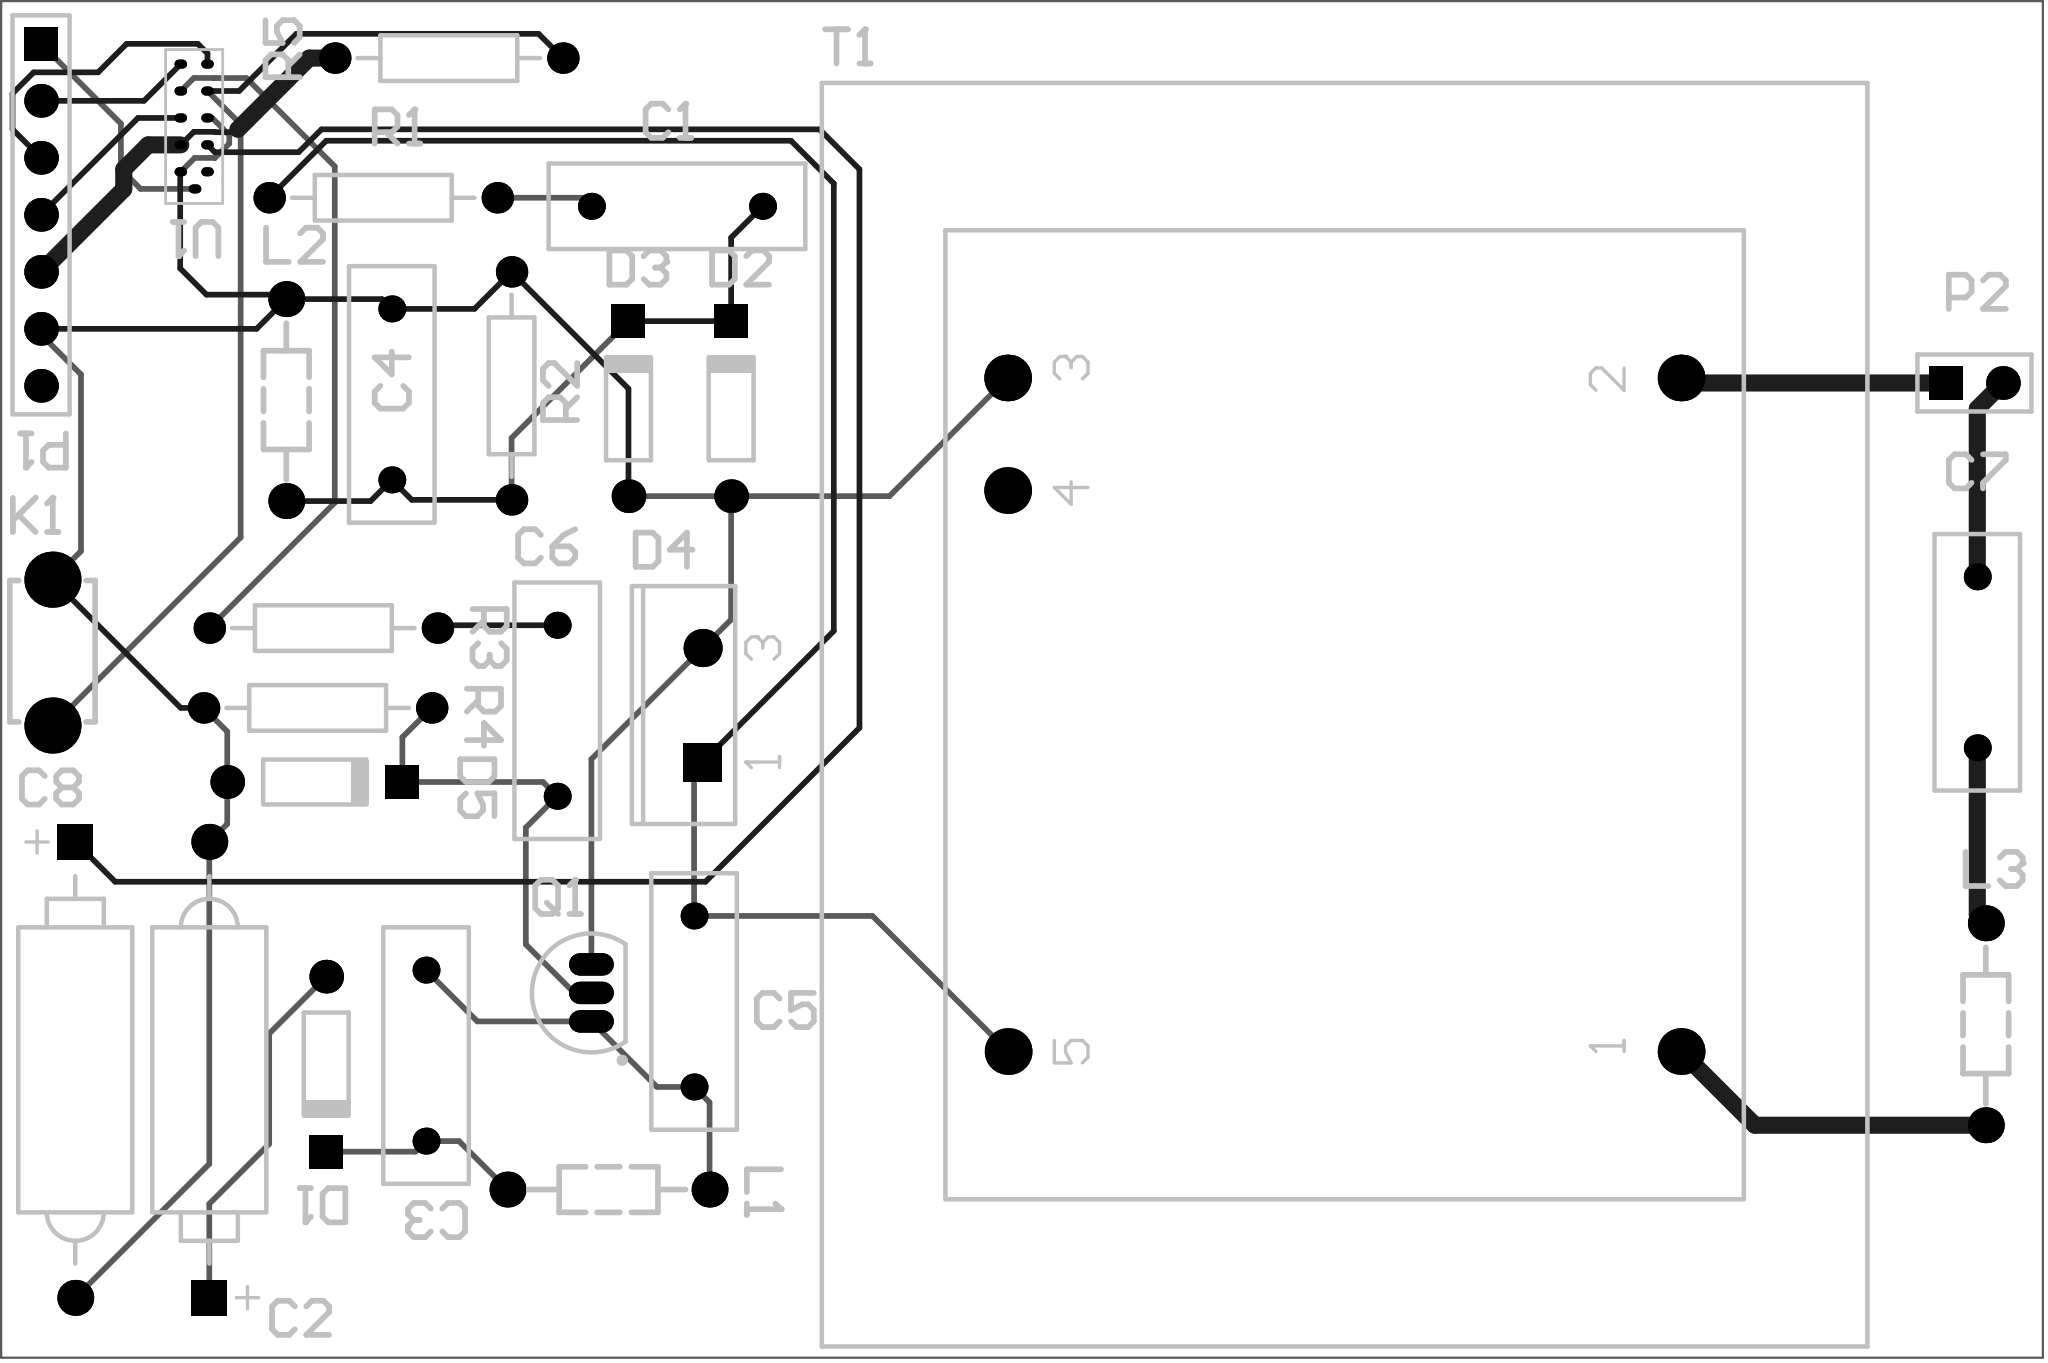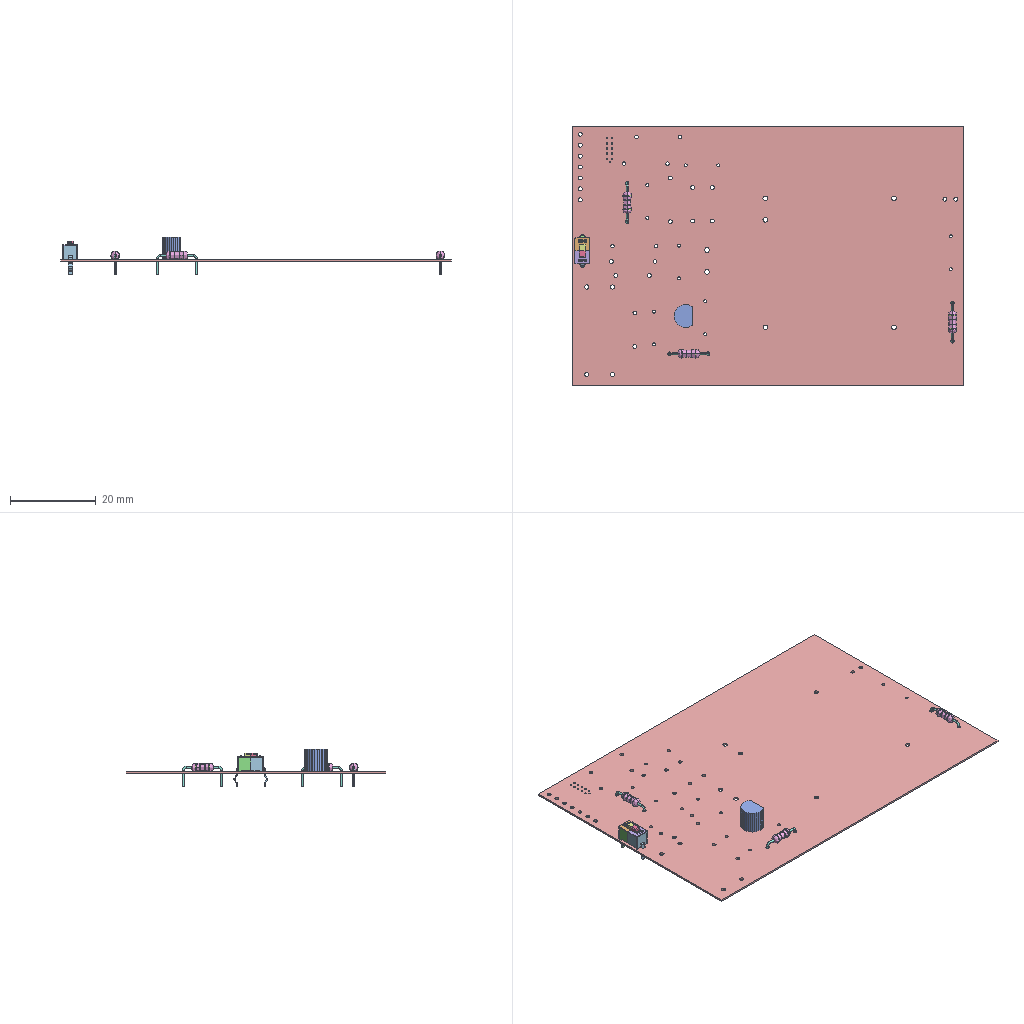Circuit board layout | Altium Designer | box 90.9 x 60.5 x 8.8 mm
Part placement:
Designator,Comment,Layer,Footprint,Center-X(mm),Center-Y(mm),Rotation
U1,KQ-330K,TopLayer,20130-10PIN,72.096,104.267,180
T1,Trans CT,TopLayer,TRF_5,123.323,78.054,90
R5,51K,TopLayer,AXIAL-0.4,83.439,107.315,180
R4,27,TopLayer,AXIAL-0.4,77.597,78.359,360
R3,27,TopLayer,AXIAL-0.4,77.851,81.915,360
R2,2.7K,TopLayer,AXIAL-0.4,86.233,92.71,270
R1,270,TopLayer,AXIAL-0.4,80.518,101.092,360
Q1,BD139,TopLayer,TO-226-AA,89.789,65.659,360
P2,CON2,TopLayer,HDR1X2,151.384,92.837,360
P1,CON7,TopLayer,HDR1X7,65.278,100.33,270
L3,15UH,TopLayer,AL0204,151.892,64.262,90
L2,220UH,TopLayer,AL0204,76.2,92.075,90
L1,68UH,TopLayer,AL0204,90.551,56.896,360
K1,KEY,TopLayer,DIP-3X6X4.3,65.786,80.824,90
D5,IN4148,TopLayer,DO-35A,77.47,75.057,360
D4,Diode 10TQ040,TopLayer,TO-220AC,94.742,78.486,90
D3,IN4148,TopLayer,DO-35A,91.44,91.694,90
D2,IN4148,TopLayer,DO-35A,96.012,91.694,90
D1,IN5819,TopLayer,DO-35A,77.978,62.484,270
C8,470UF,TopLayer,POLAR0.8,66.802,62.23,90
C7,0.1UF/250V,TopLayer,RAD-0.3,151.511,80.391,270
C6,0.33U,TopLayer,RAD-0.3,88.265,78.232,90
C5,0.033UF/50V,TopLayer,RAD-0.3,94.361,65.278,270
C4,4700P,TopLayer,RAD-0.3,80.899,92.329,90
C3,0.039UF/50V,TopLayer,RAD-0.3,82.423,62.865,270
C2,100UF/16V,TopLayer,POLAR0.8,72.771,62.23,270
C1,1500P,TopLayer,RAD-0.3,93.599,100.711,180